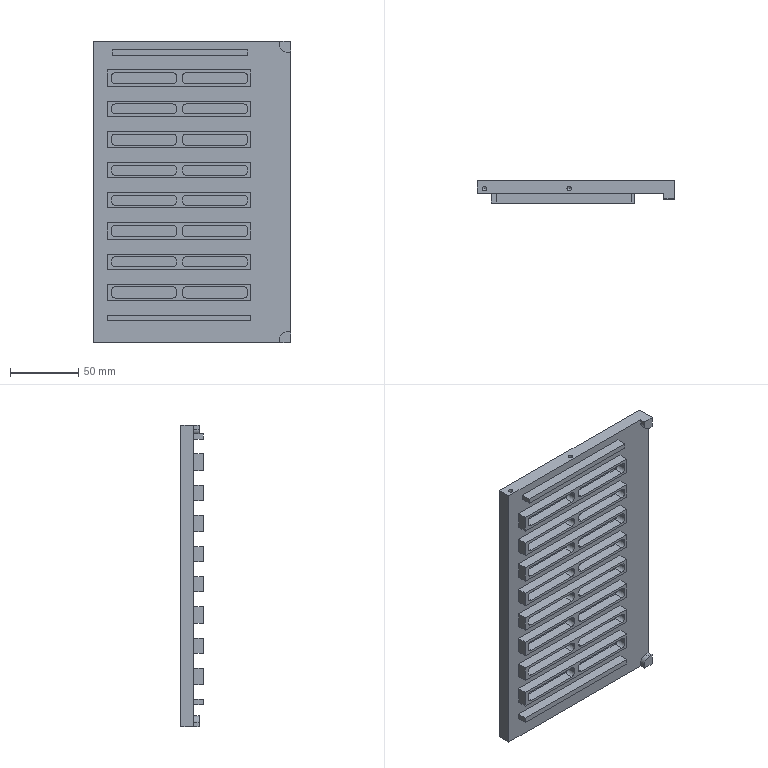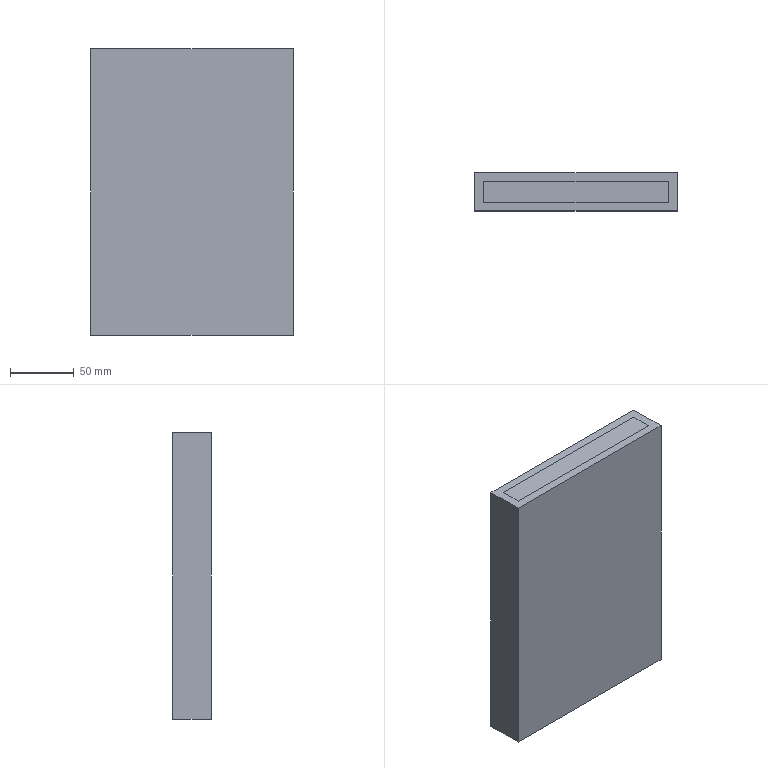CAM job | NX | 3+2 milling, drilling | part box 144.5 x 16.5 x 221 mm | stock box 158.5 x 30 x 224.5 mm
Tools:
number,name,description,diameter,corner_radius,flute_length,length,flutes
19,D8-120,Drilling Tool,8.0,0.0,35.0,50.0,2
0,D2-6-D4-50-3T-FINISH,D2-6-D4-50-3T-精,2.0,0.0,6.0,7.0,3
0,D3-9-D4-50-3T-ROUGH,D3-9-D4-50-3T,3.0,0.0,9.0,10.0,3
0,D3-9-D4-50-3T-FINISH,D3-9-D4-50-3T-精,3.0,0.0,9.0,10.0,2
3,D5-15-D6-50-3T-ROUGH,D5-15-D6-50-3T,5.0,0.0,15.0,16.0,3
5,D5-15-D6-50-3T-FINISH,D5-20-D5-75-3T,5.0,0.0,20.0,75.0,3
2,D8-25-D8-60-3T-ROUGH,D8-25-D8-60-3T-粗,8.0,0.0,25.0,60.0,2
4,D8-25-D8-60-3T-FINISH,D8-25-D8-60-3T,8.0,0.0,25.0,60.0,3
0,D10-30-D10-75-3T-ROUGH,D10-30-D10-75-3T-粗,10.0,0.0,30.0,75.0,2
4,D12-36-D12-120-3T-FINISH,D12-55-D12-120-3T,12.0,0.0,55.0,120.0,3
0,D16-48-D16-100-3T-FINISH,D16-48-D16-100-3T,16.0,0.0,48.0,100.0,3
0,刀杆C25-D25-150-2T,刀杆C25-D25-150-2T,25.0,0.0,15.0,150.0,2
1,D63面刀,D63面刀,63.0,0.0,30.0,30.0,4
9,钻头D3.3-45-73,钻刀D3.3-45-73,3.3,0.0,45.0,73.0,2
11,上排M4-13-D5-52,上排M4-13-D5-52,4.0,0.0,14.0,17.0,2
6,倒角D6-90度,倒角D6-90度,6.0,0.0,5.0,50.0,2
10,D3.3插刀,Milling Tool-5 Parameters,3.3,0.0,30.0,30.0,4
11,THREAD_MILL,Thread Mill,3.15,0.0,20.0,50.0,2
Operations:
program,operation,operation_type,tool,method,geometry_group,spindle_rpm,surface_speed,feed_per_tooth,feed_cut,feed_plunge,cut_length_mm,path_length_mm,cut_time_min,machine_time_min
A1,FLOOR_WALL,VolumeBased25DMillingOperation,D63面刀,METHOD,A-G54,3500.0,692.0,0.0714,1000.0,100.0,1321.049,1354.849,1.321,1.324
A2,动态加工0.5,CavityMilling,D8-25-D8-60-3T-ROUGH,METHOD,WORKPIECE_54,6000.0,226.0,0.2917,3500.0,100.0,39756.234,41149.964,11.189,11.328
A3,动态加工0.5_COPY_1,CavityMilling,D5-15-D6-50-3T-ROUGH,METHOD,WORKPIECE_54,5000.0,78.0,0.1,1500.0,100.0,5461.917,8816.907,2.838,3.173
A4,FLOOR_WALL_1,VolumeBased25DMillingOperation,D12-36-D12-120-3T-FINISH,METHOD,WORKPIECE_54,4000.0,150.0,0.0833,1000.0,100.0,3084.207,3132.177,3.084,3.089
A4,PLANAR_MILL,PlanarMilling,D8-25-D8-60-3T-FINISH,METHOD,WORKPIECE_54,4000.0,150.0,0.0833,1000.0,100.0,486.0,770.7,0.486,0.5145
A4,PLANAR_MILL_COPY,PlanarMilling,D8-25-D8-60-3T-FINISH,METHOD,WORKPIECE_54,4000.0,150.0,0.0833,1000.0,100.0,333.0,694.06,0.333,0.3691
A5,FLOOR_WALL_1_COPY,VolumeBased25DMillingOperation,D5-15-D6-50-3T-FINISH,METHOD,WORKPIECE_54,4000.0,150.0,0.0833,1000.0,100.0,7817.342,7868.342,7.817,7.822
A5,PLANAR_MILL_1,PlanarMilling,D5-15-D6-50-3T-FINISH,METHOD,WORKPIECE_54,3500.0,54.0,0.0762,800.0,100.0,1435.8,1486.76,1.795,1.8
A6,PLANAR_MILL_1_COPY,PlanarMilling,倒角D6-90度,METHOD,WORKPIECE_54,3500.0,54.0,0.0952,1000.0,100.0,726.604,765.604,0.7266,0.7305
A7,PLANAR_MILL_1_COPY_COPY,PlanarMilling,刀杆C25-D25-150-2T,METHOD,WORKPIECE_54,3500.0,274.0,0.1143,800.0,100.0,793.54,829.54,0.9919,0.9955
A10,ZLEVEL_PROFILE_STEEP,ZLevelMilling,D5-15-D6-50-3T-ROUGH,METHOD,A-G54,4500.0,70.0,0.1481,2000.0,100.0,1612.459,1653.489,0.8062,0.8103
B1,FLOOR_WALL_2,VolumeBased25DMillingOperation,D63面刀,METHOD,B-G55,3500.0,692.0,0.0714,1000.0,100.0,7521.296,8239.343,7.521,7.593
B1,FLOOR_WALL_2_COPY,VolumeBased25DMillingOperation,D63面刀,METHOD,B-G55,3500.0,692.0,0.0571,800.0,100.0,1231.549,1267.549,1.539,1.543
B1,CAVITY_MILL,CavityMilling,D8-25-D8-60-3T-ROUGH,METHOD,WORKPIECE_55,4500.0,113.0,0.3333,3000.0,100.0,70635.372,71315.772,23.545,23.613
B1,CAVITY_MILL_COPY,CavityMilling,D5-15-D6-50-3T-ROUGH,METHOD,WORKPIECE_55,4500.0,70.0,0.0889,1200.0,100.0,26641.923,40570.213,22.202,23.594
B1,PLANAR_MILL_4,PlanarMilling,D8-25-D8-60-3T-FINISH,METHOD,WORKPIECE_55,4200.0,105.0,0.0635,800.0,100.0,96.0,498.996,0.12,0.1603
B1,PLANAR_MILL_2_COPY_2,PlanarMilling,D8-25-D8-60-3T-FINISH,METHOD,WORKPIECE_55,4200.0,105.0,0.0952,1200.0,100.0,7245.867,7295.806,6.038,6.043
B1,PLANAR_MILL_2,PlanarMilling,D8-25-D8-60-3T-FINISH,METHOD,WORKPIECE_55,4200.0,105.0,0.0952,1200.0,100.0,2712.811,3291.851,2.261,2.319
B1,PLANAR_MILL_2_COPY_2_COPY,PlanarMilling,D8-25-D8-60-3T-FINISH,METHOD,WORKPIECE_55,4200.0,105.0,0.0635,800.0,100.0,7245.867,7295.867,9.057,9.062
B1,PLANAR_MILL_2_COPY_3,PlanarMilling,D8-25-D8-60-3T-FINISH,METHOD,WORKPIECE_55,4200.0,105.0,0.0635,800.0,100.0,2710.294,3289.974,3.388,3.446
B1,PLANAR_MILL_2_COPY,PlanarMilling,D8-25-D8-60-3T-FINISH,METHOD,WORKPIECE_55,4200.0,105.0,0.0635,800.0,100.0,60.841,353.761,0.0761,0.1053
B1,PLANAR_MILL_3,PlanarMilling,D5-15-D6-50-3T-FINISH,METHOD,WORKPIECE_55,4200.0,105.0,0.0635,800.0,100.0,1646.234,2899.787,2.058,2.183
B1,PLANAR_MILL_3_COPY,PlanarMilling,D5-15-D6-50-3T-FINISH,METHOD,WORKPIECE_55,4200.0,105.0,0.0635,800.0,100.0,1571.704,2760.26,1.965,2.083
B1,PLANAR_MILL_2_COPY_1,PlanarMilling,倒角D6-90度,METHOD,WORKPIECE_55,3500.0,65.0,0.1429,1000.0,100.0,2513.632,3124.57,2.514,2.575
B1,PLANAR_MILL_3_COPY_COPY,PlanarMilling,倒角D6-90度,METHOD,WORKPIECE_55,3500.0,65.0,0.1429,1000.0,100.0,1673.351,2691.887,1.673,1.775
C1,DRILLING,Operation,D8-120,METHOD,C-G56,2000.0,37.0,0.05,200.0,0.0,15.6,281.401,0.078,0.1046
C1,DRILLING_COPY,Operation,钻头D3.3-45-73,METHOD,C-G56,2000.0,37.0,0.05,200.0,0.0,49.8,349.801,0.249,0.279
C1,DRILLING_COPY_COPY,Operation,D3.3插刀,METHOD,C-G56,2000.0,37.0,0.05,200.0,0.0,50.0,350.202,0.25,0.28
C1,THREAD_MILLING,ThreadMilling,THREAD_MILL,METHOD,C-G56,3000.0,29.0,0.0333,200.0,100.0,254.875,747.579,1.274,1.324
C9,DRILLING_COPY_COPY_COPY,Operation,上排M4-13-D5-52,METHOD,C-G56,2000.0,37.0,0.05,200.0,0.0,48.8,347.801,0.244,0.2739
D1,DRILLING_COPY_1,Operation,倒角D6-90度,METHOD,D-G57,2000.0,37.0,0.0375,150.0,0.0,7.8,120.672,0.052,0.0633
D1,DRILLING_COPY_COPY_1,Operation,钻头D3.3-45-73,METHOD,D-G57,2000.0,37.0,0.05,200.0,0.0,25.8,156.673,0.129,0.1421
D1,PLANAR_MILL_9_COPY,PlanarMilling,D2-6-D4-50-3T-FINISH,METHOD,D-G57,4500.0,28.0,0.0444,600.0,100.0,262.59,421.406,0.4376,0.4535
D1,THREAD_MILLING_2,ThreadMilling,THREAD_MILL,METHOD,D-G57,4500.0,44.0,0.0167,150.0,100.0,129.445,342.868,0.863,0.8843
D1,PLANAR_MILL_10_COPY_1,PlanarMilling,D16-48-D16-100-3T-FINISH,METHOD,D-G57,3500.0,175.0,0.0762,800.0,100.0,182.5,216.44,0.2281,0.2315
D1,PLANAR_MILL_10_COPY_1_COPY,PlanarMilling,D16-48-D16-100-3T-FINISH,METHOD,D-G57,3500.0,175.0,0.0762,800.0,100.0,182.5,216.5,0.2281,0.2315
E1,DRILLING_COPY_1_COPY,Operation,倒角D6-90度,METHOD,E-G58,2000.0,37.0,0.0375,150.0,0.0,7.8,140.673,0.052,0.0653
E1,DRILLING_COPY_COPY_1_COPY,Operation,钻头D3.3-45-73,METHOD,E-G58,2000.0,37.0,0.05,200.0,0.0,25.8,176.673,0.129,0.1441
E1,PLANAR_MILL_9,PlanarMilling,D2-6-D4-50-3T-FINISH,METHOD,E-G58,4500.0,28.0,0.0444,600.0,100.0,262.59,461.08,0.4376,0.4575
E1,THREAD_MILLING_1,ThreadMilling,THREAD_MILL,METHOD,E-G58,4500.0,44.0,0.0167,150.0,100.0,158.081,418.075,1.054,1.08
E1,PLANAR_MILL_10,PlanarMilling,D16-48-D16-100-3T-FINISH,METHOD,E-G58,3500.0,175.0,0.0762,800.0,100.0,182.5,236.44,0.2281,0.2335
E1,PLANAR_MILL_10_COPY,PlanarMilling,D16-48-D16-100-3T-FINISH,METHOD,E-G58,3500.0,175.0,0.0762,800.0,100.0,182.5,236.5,0.2281,0.2335
G1,PLANAR_MILL_5,PlanarMilling,D8-25-D8-60-3T-ROUGH,METHOD,F-G59,4500.0,113.0,0.1111,1000.0,100.0,447.931,1193.949,0.4479,0.5225
G1,PLANAR_MILL_5_COPY,PlanarMilling,D8-25-D8-60-3T-FINISH,METHOD,F-G59,4500.0,113.0,0.1111,1000.0,100.0,449.702,1195.8,0.4497,0.5243
G1,PLANAR_MILL_6,PlanarMilling,D3-9-D4-50-3T-FINISH,METHOD,F-G59,4500.0,42.0,0.0889,800.0,100.0,136.272,858.771,0.1703,0.2426
工装1,PLANAR_MILL_COPY_1,PlanarMilling,D8-25-D8-60-3T-FINISH,METHOD,WORKPIECE_54,4000.0,100.0,0.05,600.0,100.0,486.0,770.5,0.81,0.8384
工装1,PLANAR_MILL_COPY_COPY,PlanarMilling,D8-25-D8-60-3T-FINISH,METHOD,WORKPIECE_54,4000.0,150.0,0.0833,1000.0,100.0,333.0,694.06,0.333,0.3691
工装4,PLANAR_MILL_8,PlanarMilling,D8-25-D8-60-3T-ROUGH,METHOD,GZ4,4500.0,113.0,0.1111,1000.0,100.0,7496.276,8002.276,7.496,7.547
工装4,PLANAR_MILL_8_COPY,PlanarMilling,D5-15-D6-50-3T-ROUGH,METHOD,GZ4,4500.0,113.0,0.1111,1000.0,100.0,2104.623,5367.314,2.105,2.431
工装4,PLANAR_MILL_8_COPY_1,PlanarMilling,D3-9-D4-50-3T-ROUGH,METHOD,GZ4,4500.0,70.0,0.0593,800.0,100.0,749.704,803.704,0.9371,0.9425
工装4,PLANAR_MILL_8_COPY_1_COPY,PlanarMilling,倒角D6-90度,METHOD,GZ4,4500.0,70.0,0.0593,800.0,100.0,761.984,800.984,0.9525,0.9564
工装5,PLANAR_MILL_7,PlanarMilling,D10-30-D10-75-3T-ROUGH,METHOD,GZ5,4500.0,141.0,0.1111,1000.0,100.0,1566.0,2968.0,1.566,1.706